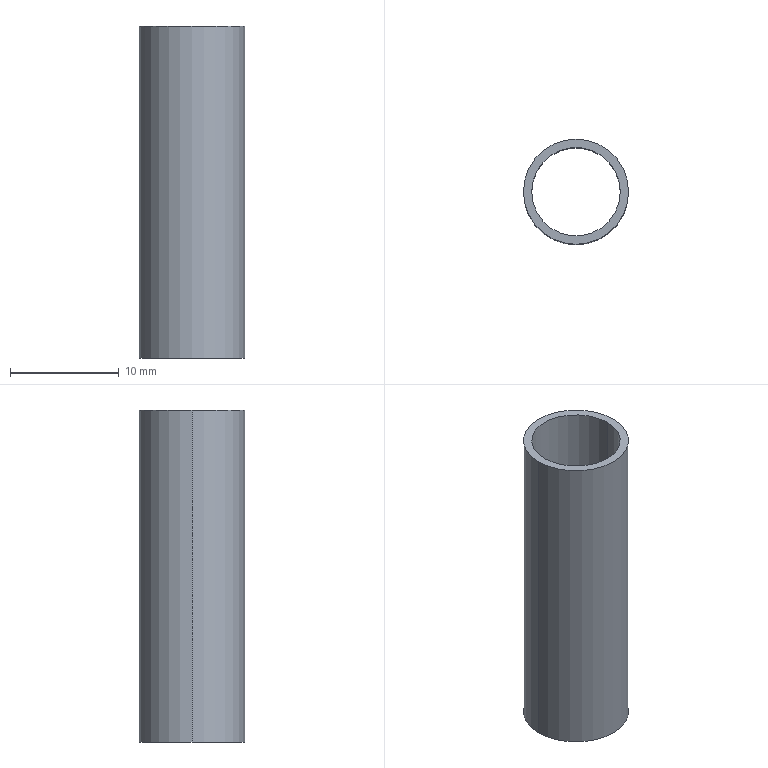Part | SolidWorks | features Extrusion 1, Scale 1 | 1 solid | 6 faces | box 9.652 x 9.652 x 30.48 mm | volume 648.667 mm3 | cylinder 4 | plane 2 | commonest cylinder face diameters 8.128 x2 9.652 x2
STEP:
#1=CARTESIAN_POINT('',(-4.064,0.,-30.48));
#2=VERTEX_POINT('',#1);
#3=CARTESIAN_POINT('',(4.064,0.,-30.48));
#4=VERTEX_POINT('',#3);
#5=CARTESIAN_POINT('',(0.,0.,-30.48));
#6=DIRECTION('',(0.,0.,1.));
#7=DIRECTION('',(1.,0.,0.));
#8=AXIS2_PLACEMENT_3D('',#5,#6,#7);
#9=CIRCLE('',#8,4.064);
#10=EDGE_CURVE('',#2,#4,#9,.T.);
#11=ORIENTED_EDGE('',*,*,#10,.F.);
#12=CARTESIAN_POINT('',(-4.064,0.,0.));
#13=VERTEX_POINT('',#12);
#14=CARTESIAN_POINT('',(-4.064,0.,-30.48));
#15=DIRECTION('',(0.,0.,1.));
#16=VECTOR('',#15,1000.);
#17=LINE('',#14,#16);
#18=EDGE_CURVE('',#2,#13,#17,.T.);
#19=ORIENTED_EDGE('',*,*,#18,.T.);
#20=CARTESIAN_POINT('',(4.064,0.,0.));
#21=VERTEX_POINT('',#20);
#22=CARTESIAN_POINT('',(0.,0.,0.));
#23=DIRECTION('',(0.,0.,1.));
#24=DIRECTION('',(1.,0.,0.));
#25=AXIS2_PLACEMENT_3D('',#22,#23,#24);
#26=CIRCLE('',#25,4.064);
#27=EDGE_CURVE('',#13,#21,#26,.T.);
#28=ORIENTED_EDGE('',*,*,#27,.T.);
#29=CARTESIAN_POINT('',(4.064,0.,-30.48));
#30=DIRECTION('',(0.,0.,1.));
#31=VECTOR('',#30,1000.);
#32=LINE('',#29,#31);
#33=EDGE_CURVE('',#4,#21,#32,.T.);
#34=ORIENTED_EDGE('',*,*,#33,.F.);
#35=EDGE_LOOP('',(#11,#19,#28,#34));
#36=FACE_OUTER_BOUND('',#35,.T.);
#37=CARTESIAN_POINT('',(0.,0.,-30.48));
#38=DIRECTION('',(0.,0.,1.));
#39=DIRECTION('',(1.,0.,0.));
#40=AXIS2_PLACEMENT_3D('',#37,#38,#39);
#41=CYLINDRICAL_SURFACE('',#40,4.064);
#42=ADVANCED_FACE('',(#36),#41,.F.);
#43=CARTESIAN_POINT('',(4.826,0.,-30.48));
#44=VERTEX_POINT('',#43);
#45=CARTESIAN_POINT('',(-4.826,0.,-30.48));
#46=VERTEX_POINT('',#45);
#47=CARTESIAN_POINT('',(0.,0.,-30.48));
#48=DIRECTION('',(0.,0.,1.));
#49=DIRECTION('',(1.,0.,0.));
#50=AXIS2_PLACEMENT_3D('',#47,#48,#49);
#51=CIRCLE('',#50,4.826);
#52=EDGE_CURVE('',#44,#46,#51,.T.);
#53=ORIENTED_EDGE('',*,*,#52,.T.);
#54=CARTESIAN_POINT('',(-4.826,0.,0.));
#55=VERTEX_POINT('',#54);
#56=CARTESIAN_POINT('',(-4.826,0.,-30.48));
#57=DIRECTION('',(0.,0.,1.));
#58=VECTOR('',#57,1000.);
#59=LINE('',#56,#58);
#60=EDGE_CURVE('',#46,#55,#59,.T.);
#61=ORIENTED_EDGE('',*,*,#60,.T.);
#62=CARTESIAN_POINT('',(4.826,0.,0.));
#63=VERTEX_POINT('',#62);
#64=CARTESIAN_POINT('',(0.,0.,0.));
#65=DIRECTION('',(0.,0.,1.));
#66=DIRECTION('',(1.,0.,0.));
#67=AXIS2_PLACEMENT_3D('',#64,#65,#66);
#68=CIRCLE('',#67,4.826);
#69=EDGE_CURVE('',#63,#55,#68,.T.);
#70=ORIENTED_EDGE('',*,*,#69,.F.);
#71=CARTESIAN_POINT('',(4.826,0.,-30.48));
#72=DIRECTION('',(0.,0.,1.));
#73=VECTOR('',#72,1000.);
#74=LINE('',#71,#73);
#75=EDGE_CURVE('',#44,#63,#74,.T.);
#76=ORIENTED_EDGE('',*,*,#75,.F.);
#77=EDGE_LOOP('',(#53,#61,#70,#76));
#78=FACE_OUTER_BOUND('',#77,.T.);
#79=CARTESIAN_POINT('',(0.,0.,-30.48));
#80=DIRECTION('',(0.,0.,1.));
#81=DIRECTION('',(1.,0.,0.));
#82=AXIS2_PLACEMENT_3D('',#79,#80,#81);
#83=CYLINDRICAL_SURFACE('',#82,4.826);
#84=ADVANCED_FACE('',(#78),#83,.T.);
#85=ORIENTED_EDGE('',*,*,#60,.F.);
#86=CARTESIAN_POINT('',(0.,0.,-30.48));
#87=DIRECTION('',(0.,0.,1.));
#88=DIRECTION('',(1.,0.,0.));
#89=AXIS2_PLACEMENT_3D('',#86,#87,#88);
#90=CIRCLE('',#89,4.826);
#91=EDGE_CURVE('',#46,#44,#90,.T.);
#92=ORIENTED_EDGE('',*,*,#91,.T.);
#93=ORIENTED_EDGE('',*,*,#75,.T.);
#94=CARTESIAN_POINT('',(0.,0.,0.));
#95=DIRECTION('',(0.,0.,1.));
#96=DIRECTION('',(1.,0.,0.));
#97=AXIS2_PLACEMENT_3D('',#94,#95,#96);
#98=CIRCLE('',#97,4.826);
#99=EDGE_CURVE('',#55,#63,#98,.T.);
#100=ORIENTED_EDGE('',*,*,#99,.F.);
#101=EDGE_LOOP('',(#85,#92,#93,#100));
#102=FACE_OUTER_BOUND('',#101,.T.);
#103=CARTESIAN_POINT('',(0.,0.,-30.48));
#104=DIRECTION('',(0.,0.,1.));
#105=DIRECTION('',(1.,0.,0.));
#106=AXIS2_PLACEMENT_3D('',#103,#104,#105);
#107=CYLINDRICAL_SURFACE('',#106,4.826);
#108=ADVANCED_FACE('',(#102),#107,.T.);
#109=CARTESIAN_POINT('',(0.,0.,-30.48));
#110=DIRECTION('',(0.,0.,1.));
#111=DIRECTION('',(1.,0.,0.));
#112=AXIS2_PLACEMENT_3D('',#109,#110,#111);
#113=CIRCLE('',#112,4.064);
#114=EDGE_CURVE('',#4,#2,#113,.T.);
#115=ORIENTED_EDGE('',*,*,#114,.T.);
#116=ORIENTED_EDGE('',*,*,#10,.T.);
#117=EDGE_LOOP('',(#115,#116));
#118=FACE_BOUND('',#117,.T.);
#119=ORIENTED_EDGE('',*,*,#52,.F.);
#120=ORIENTED_EDGE('',*,*,#91,.F.);
#121=EDGE_LOOP('',(#119,#120));
#122=FACE_OUTER_BOUND('',#121,.T.);
#123=CARTESIAN_POINT('',(0.,0.,-30.48));
#124=DIRECTION('',(0.,0.,1.));
#125=DIRECTION('',(1.,0.,0.));
#126=AXIS2_PLACEMENT_3D('',#123,#124,#125);
#127=PLANE('',#126);
#128=ADVANCED_FACE('',(#118,#122),#127,.F.);
#129=CARTESIAN_POINT('',(0.,0.,0.));
#130=DIRECTION('',(0.,0.,1.));
#131=DIRECTION('',(1.,0.,0.));
#132=AXIS2_PLACEMENT_3D('',#129,#130,#131);
#133=CIRCLE('',#132,4.064);
#134=EDGE_CURVE('',#21,#13,#133,.T.);
#135=ORIENTED_EDGE('',*,*,#134,.F.);
#136=ORIENTED_EDGE('',*,*,#27,.F.);
#137=EDGE_LOOP('',(#135,#136));
#138=FACE_BOUND('',#137,.T.);
#139=ORIENTED_EDGE('',*,*,#69,.T.);
#140=ORIENTED_EDGE('',*,*,#99,.T.);
#141=EDGE_LOOP('',(#139,#140));
#142=FACE_OUTER_BOUND('',#141,.T.);
#143=CARTESIAN_POINT('',(0.,0.,0.));
#144=DIRECTION('',(0.,0.,1.));
#145=DIRECTION('',(1.,0.,0.));
#146=AXIS2_PLACEMENT_3D('',#143,#144,#145);
#147=PLANE('',#146);
#148=ADVANCED_FACE('',(#138,#142),#147,.T.);
#149=ORIENTED_EDGE('',*,*,#18,.F.);
#150=ORIENTED_EDGE('',*,*,#114,.F.);
#151=ORIENTED_EDGE('',*,*,#33,.T.);
#152=ORIENTED_EDGE('',*,*,#134,.T.);
#153=EDGE_LOOP('',(#149,#150,#151,#152));
#154=FACE_OUTER_BOUND('',#153,.T.);
#155=CARTESIAN_POINT('',(0.,0.,-30.48));
#156=DIRECTION('',(0.,0.,1.));
#157=DIRECTION('',(1.,0.,0.));
#158=AXIS2_PLACEMENT_3D('',#155,#156,#157);
#159=CYLINDRICAL_SURFACE('',#158,4.064);
#160=ADVANCED_FACE('',(#154),#159,.F.);
#161=CLOSED_SHELL('',(#42,#84,#108,#128,#148,#160));
#162=MANIFOLD_SOLID_BREP('',#161);
#163=CARTESIAN_POINT('',(0.,0.,0.));
#164=DIRECTION('',(0.,0.,1.));
#165=DIRECTION('',(1.,0.,0.));
#166=AXIS2_PLACEMENT_3D('',#163,#164,#165);
#167=(LENGTH_UNIT()NAMED_UNIT(*)SI_UNIT(.MILLI.,.METRE.));
#168=UNCERTAINTY_MEASURE_WITH_UNIT(LENGTH_MEASURE(0.00001),#167,'','');
#169=(NAMED_UNIT(*)PLANE_ANGLE_UNIT()SI_UNIT($,.RADIAN.));
#170=(NAMED_UNIT(*)SI_UNIT($,.STERADIAN.)SOLID_ANGLE_UNIT());
#171=(GEOMETRIC_REPRESENTATION_CONTEXT(3)GLOBAL_UNCERTAINTY_ASSIGNED_CONTEXT((#168))GLOBAL_UNIT_ASSIGNED_CONTEXT((#167,#169,#170))REPRESENTATION_CONTEXT('',''));
#172=ADVANCED_BREP_SHAPE_REPRESENTATION('',(#162,#166),#171);